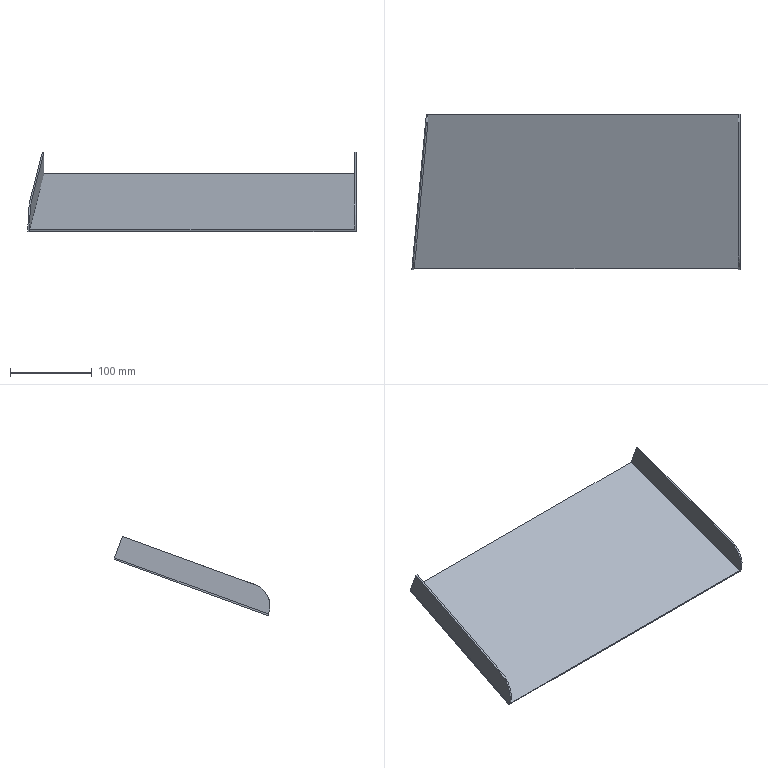Part | NX | features solid 2 | 1 solid | 16 faces | box 400.679 x 190.481 x 96.654 mm | volume 178538 mm3 | plane 11 | spline 3 | cylinder 2 | commonest cylinder face diameters 56 x2
STEP:
#1=CARTESIAN_POINT('',(-874.402,-997.254,-367.866));
#2=VERTEX_POINT('',#1);
#3=CARTESIAN_POINT('',(-475.731,-997.254,-367.866));
#4=VERTEX_POINT('',#3);
#5=CARTESIAN_POINT('',(-849.475,-997.254,-367.866));
#6=DIRECTION('',(-1.,0.,0.));
#7=VECTOR('',#6,1000.);
#8=LINE('',#5,#7);
#9=EDGE_CURVE('',#2,#4,#8,.F.);
#10=ORIENTED_EDGE('',*,*,#9,.T.);
#11=CARTESIAN_POINT('',(-475.731,-997.939,-365.986));
#12=VERTEX_POINT('',#11);
#13=CARTESIAN_POINT('',(-475.731,-997.254,-367.866));
#14=DIRECTION('',(0.,-0.342,0.9397));
#15=VECTOR('',#14,1000.);
#16=LINE('',#13,#15);
#17=EDGE_CURVE('',#4,#12,#16,.T.);
#18=ORIENTED_EDGE('',*,*,#17,.T.);
#19=CARTESIAN_POINT('',(-477.731,-997.939,-365.986));
#20=VERTEX_POINT('',#19);
#21=CARTESIAN_POINT('',(-475.731,-997.939,-365.986));
#22=DIRECTION('',(-1.,0.,0.));
#23=VECTOR('',#22,1000.);
#24=LINE('',#21,#23);
#25=EDGE_CURVE('',#12,#20,#24,.T.);
#26=ORIENTED_EDGE('',*,*,#25,.T.);
#27=CARTESIAN_POINT('',(-874.402,-997.939,-365.986));
#28=VERTEX_POINT('',#27);
#29=CARTESIAN_POINT('',(-849.475,-997.939,-365.986));
#30=DIRECTION('',(-1.,0.,0.));
#31=VECTOR('',#30,1000.);
#32=LINE('',#29,#31);
#33=EDGE_CURVE('',#28,#20,#32,.F.);
#34=ORIENTED_EDGE('',*,*,#33,.F.);
#35=CARTESIAN_POINT('',(-874.402,-997.254,-367.866));
#36=DIRECTION('',(0.,-0.342,0.9397));
#37=VECTOR('',#36,1000.);
#38=LINE('',#35,#37);
#39=EDGE_CURVE('',#28,#2,#38,.F.);
#40=ORIENTED_EDGE('',*,*,#39,.T.);
#41=EDGE_LOOP('',(#10,#18,#26,#34,#40));
#42=FACE_BOUND('',#41,.T.);
#43=CARTESIAN_POINT('',(-849.475,-997.254,-367.866));
#44=DIRECTION('',(0.,0.9397,0.342));
#45=DIRECTION('',(1.,0.,0.));
#46=AXIS2_PLACEMENT_3D('',#43,#44,#45);
#47=PLANE('',#46);
#48=ADVANCED_FACE('',(#42),#47,.F.);
#49=CARTESIAN_POINT('',(-858.894,-810.,-297.582));
#50=VERTEX_POINT('',#49);
#51=CARTESIAN_POINT('',(-477.731,-810.,-297.582));
#52=VERTEX_POINT('',#51);
#53=CARTESIAN_POINT('',(-849.475,-810.,-297.582));
#54=DIRECTION('',(1.,0.,0.));
#55=VECTOR('',#54,1000.);
#56=LINE('',#53,#55);
#57=EDGE_CURVE('',#50,#52,#56,.T.);
#58=ORIENTED_EDGE('',*,*,#57,.T.);
#59=CARTESIAN_POINT('',(-477.731,-819.577,-271.271));
#60=VERTEX_POINT('',#59);
#61=CARTESIAN_POINT('',(-477.731,-809.316,-299.462));
#62=DIRECTION('',(0.,-0.342,0.9397));
#63=VECTOR('',#62,1000.);
#64=LINE('',#61,#63);
#65=EDGE_CURVE('',#52,#60,#64,.T.);
#66=ORIENTED_EDGE('',*,*,#65,.T.);
#67=CARTESIAN_POINT('',(-475.731,-819.577,-271.271));
#68=VERTEX_POINT('',#67);
#69=CARTESIAN_POINT('',(-475.731,-819.577,-271.271));
#70=DIRECTION('',(1.,0.,0.));
#71=VECTOR('',#70,1000.);
#72=LINE('',#69,#71);
#73=EDGE_CURVE('',#68,#60,#72,.F.);
#74=ORIENTED_EDGE('',*,*,#73,.F.);
#75=CARTESIAN_POINT('',(-475.731,-809.316,-299.462));
#76=VERTEX_POINT('',#75);
#77=CARTESIAN_POINT('',(-475.731,-891.114,-74.722));
#78=DIRECTION('',(0.,0.342,-0.9397));
#79=VECTOR('',#78,1000.);
#80=LINE('',#77,#79);
#81=EDGE_CURVE('',#76,#68,#80,.F.);
#82=ORIENTED_EDGE('',*,*,#81,.F.);
#83=CARTESIAN_POINT('',(-858.894,-809.316,-299.462));
#84=VERTEX_POINT('',#83);
#85=CARTESIAN_POINT('',(-849.475,-809.316,-299.462));
#86=DIRECTION('',(1.,0.,0.));
#87=VECTOR('',#86,1000.);
#88=LINE('',#85,#87);
#89=EDGE_CURVE('',#84,#76,#88,.T.);
#90=ORIENTED_EDGE('',*,*,#89,.F.);
#91=CARTESIAN_POINT('',(-858.894,-809.658,-298.522));
#92=DIRECTION('',(0.,-0.342,0.9397));
#93=VECTOR('',#92,1000.);
#94=LINE('',#91,#93);
#95=EDGE_CURVE('',#84,#50,#94,.T.);
#96=ORIENTED_EDGE('',*,*,#95,.T.);
#97=EDGE_LOOP('',(#58,#66,#74,#82,#90,#96));
#98=FACE_BOUND('',#97,.T.);
#99=CARTESIAN_POINT('',(-849.475,-809.316,-299.462));
#100=DIRECTION('',(0.,0.9397,0.342));
#101=DIRECTION('',(1.,0.,0.));
#102=AXIS2_PLACEMENT_3D('',#99,#100,#101);
#103=PLANE('',#102);
#104=ADVANCED_FACE('',(#98),#103,.T.);
#105=ORIENTED_EDGE('',*,*,#95,.F.);
#106=CARTESIAN_POINT('',(-876.41,-997.254,-367.866));
#107=VERTEX_POINT('',#106);
#108=CARTESIAN_POINT('',(-858.894,-809.316,-299.462));
#109=CARTESIAN_POINT('',(-864.732,-871.962,-322.263));
#110=CARTESIAN_POINT('',(-870.571,-934.608,-345.064));
#111=CARTESIAN_POINT('',(-876.41,-997.254,-367.866));
#112=B_SPLINE_CURVE_WITH_KNOTS('',3,(#108,#109,#110,#111),.UNSPECIFIED.,.F.,.F.,(4,4),(-0.03011,0.1707),.UNSPECIFIED.);
#113=EDGE_CURVE('',#84,#107,#112,.T.);
#114=ORIENTED_EDGE('',*,*,#113,.T.);
#115=CARTESIAN_POINT('',(-876.41,-997.939,-365.986));
#116=VERTEX_POINT('',#115);
#117=CARTESIAN_POINT('',(-876.41,-997.597,-366.926));
#118=DIRECTION('',(0.,-0.342,0.9397));
#119=VECTOR('',#118,1000.);
#120=LINE('',#117,#119);
#121=EDGE_CURVE('',#107,#116,#120,.T.);
#122=ORIENTED_EDGE('',*,*,#121,.T.);
#123=CARTESIAN_POINT('',(-876.41,-997.939,-365.986));
#124=CARTESIAN_POINT('',(-870.571,-935.292,-343.185));
#125=CARTESIAN_POINT('',(-864.732,-872.646,-320.384));
#126=CARTESIAN_POINT('',(-858.894,-810.,-297.582));
#127=B_SPLINE_CURVE_WITH_KNOTS('',3,(#123,#124,#125,#126),.UNSPECIFIED.,.F.,.F.,(4,4),(0.6901,0.8909),.UNSPECIFIED.);
#128=EDGE_CURVE('',#50,#116,#127,.F.);
#129=ORIENTED_EDGE('',*,*,#128,.F.);
#130=EDGE_LOOP('',(#105,#114,#122,#129));
#131=FACE_BOUND('',#130,.T.);
#132=CARTESIAN_POINT('',(-858.894,-809.316,-299.462));
#133=CARTESIAN_POINT('',(-858.894,-810.,-297.582));
#134=CARTESIAN_POINT('',(-864.732,-871.962,-322.263));
#135=CARTESIAN_POINT('',(-864.732,-872.646,-320.384));
#136=CARTESIAN_POINT('',(-870.571,-934.608,-345.064));
#137=CARTESIAN_POINT('',(-870.571,-935.292,-343.185));
#138=CARTESIAN_POINT('',(-876.41,-997.254,-367.866));
#139=CARTESIAN_POINT('',(-876.41,-997.939,-365.986));
#140=B_SPLINE_SURFACE_WITH_KNOTS('',3,1,((#132,#133),(#134,#135),(#136,#137),(#138,#139)),.SURF_OF_LINEAR_EXTRUSION.,.F.,.F.,.F.,(4,4),(2,2),(0.,1.),(0.,1.),.PIECEWISE_BEZIER_KNOTS.);
#141=ADVANCED_FACE('',(#131),#140,.T.);
#142=ORIENTED_EDGE('',*,*,#33,.T.);
#143=CARTESIAN_POINT('',(-477.731,-838.191,-307.843));
#144=DIRECTION('',(0.,0.9397,0.342));
#145=VECTOR('',#144,1000.);
#146=LINE('',#143,#145);
#147=EDGE_CURVE('',#20,#52,#146,.T.);
#148=ORIENTED_EDGE('',*,*,#147,.T.);
#149=ORIENTED_EDGE('',*,*,#57,.F.);
#150=CARTESIAN_POINT('',(-856.901,-810.164,-297.642));
#151=VERTEX_POINT('',#150);
#152=CARTESIAN_POINT('',(-846.94,-810.984,-297.94));
#153=DIRECTION('',(-0.9962,0.08198,0.02984));
#154=VECTOR('',#153,1000.);
#155=LINE('',#152,#154);
#156=EDGE_CURVE('',#50,#151,#155,.F.);
#157=ORIENTED_EDGE('',*,*,#156,.T.);
#158=CARTESIAN_POINT('',(-859.437,-837.371,-307.545));
#159=DIRECTION('',(0.08725,0.9361,0.3407));
#160=VECTOR('',#159,1000.);
#161=LINE('',#158,#160);
#162=EDGE_CURVE('',#28,#151,#161,.T.);
#163=ORIENTED_EDGE('',*,*,#162,.F.);
#164=EDGE_LOOP('',(#142,#148,#149,#157,#163));
#165=FACE_BOUND('',#164,.T.);
#166=CARTESIAN_POINT('',(-849.475,-838.191,-307.843));
#167=DIRECTION('',(0.,0.342,-0.9397));
#168=DIRECTION('',(-1.,0.,0.));
#169=AXIS2_PLACEMENT_3D('',#166,#167,#168);
#170=PLANE('',#169);
#171=ADVANCED_FACE('',(#165),#170,.F.);
#172=CARTESIAN_POINT('',(-475.731,-837.507,-309.722));
#173=DIRECTION('',(0.,0.9397,0.342));
#174=VECTOR('',#173,1000.);
#175=LINE('',#172,#174);
#176=EDGE_CURVE('',#76,#4,#175,.F.);
#177=ORIENTED_EDGE('',*,*,#176,.F.);
#178=ORIENTED_EDGE('',*,*,#81,.T.);
#179=CARTESIAN_POINT('',(-475.731,-981.204,-330.098));
#180=VERTEX_POINT('',#179);
#181=CARTESIAN_POINT('',(-475.731,-819.577,-271.271));
#182=DIRECTION('',(0.,-0.9397,-0.342));
#183=VECTOR('',#182,1000.);
#184=LINE('',#181,#183);
#185=EDGE_CURVE('',#68,#180,#184,.T.);
#186=ORIENTED_EDGE('',*,*,#185,.T.);
#187=CARTESIAN_POINT('',(-475.731,-971.627,-356.41));
#188=DIRECTION('',(-1.,0.,0.));
#189=DIRECTION('',(0.,-1.,0.));
#190=AXIS2_PLACEMENT_3D('',#187,#188,#189);
#191=CIRCLE('',#190,28.);
#192=EDGE_CURVE('',#180,#12,#191,.F.);
#193=ORIENTED_EDGE('',*,*,#192,.T.);
#194=ORIENTED_EDGE('',*,*,#17,.F.);
#195=EDGE_LOOP('',(#177,#178,#186,#193,#194));
#196=FACE_BOUND('',#195,.T.);
#197=CARTESIAN_POINT('',(-475.731,-608.443,28.162));
#198=DIRECTION('',(-1.,0.,0.));
#199=DIRECTION('',(0.,-0.9397,-0.342));
#200=AXIS2_PLACEMENT_3D('',#197,#198,#199);
#201=PLANE('',#200);
#202=ADVANCED_FACE('',(#196),#201,.F.);
#203=ORIENTED_EDGE('',*,*,#89,.T.);
#204=ORIENTED_EDGE('',*,*,#176,.T.);
#205=ORIENTED_EDGE('',*,*,#9,.F.);
#206=CARTESIAN_POINT('',(-876.41,-997.254,-367.866));
#207=VERTEX_POINT('',#206);
#208=CARTESIAN_POINT('',(-849.475,-997.254,-367.866));
#209=DIRECTION('',(-1.,0.,0.));
#210=VECTOR('',#209,1000.);
#211=LINE('',#208,#210);
#212=EDGE_CURVE('',#207,#2,#211,.F.);
#213=ORIENTED_EDGE('',*,*,#212,.F.);
#214=CARTESIAN_POINT('',(-849.475,-997.254,-367.866));
#215=DIRECTION('',(-1.,0.,0.));
#216=VECTOR('',#215,1000.);
#217=LINE('',#214,#216);
#218=EDGE_CURVE('',#107,#207,#217,.F.);
#219=ORIENTED_EDGE('',*,*,#218,.F.);
#220=ORIENTED_EDGE('',*,*,#113,.F.);
#221=EDGE_LOOP('',(#203,#204,#205,#213,#219,#220));
#222=FACE_BOUND('',#221,.T.);
#223=CARTESIAN_POINT('',(-849.475,-837.507,-309.722));
#224=DIRECTION('',(0.,0.342,-0.9397));
#225=DIRECTION('',(-1.,0.,0.));
#226=AXIS2_PLACEMENT_3D('',#223,#224,#225);
#227=PLANE('',#226);
#228=ADVANCED_FACE('',(#222),#227,.T.);
#229=ORIENTED_EDGE('',*,*,#156,.F.);
#230=CARTESIAN_POINT('',(-858.894,-819.577,-271.271));
#231=VERTEX_POINT('',#230);
#232=CARTESIAN_POINT('',(-858.894,-809.316,-299.462));
#233=DIRECTION('',(0.,-0.342,0.9397));
#234=VECTOR('',#233,1000.);
#235=LINE('',#232,#234);
#236=EDGE_CURVE('',#50,#231,#235,.T.);
#237=ORIENTED_EDGE('',*,*,#236,.T.);
#238=CARTESIAN_POINT('',(-856.901,-819.741,-271.331));
#239=VERTEX_POINT('',#238);
#240=CARTESIAN_POINT('',(-858.894,-819.577,-271.271));
#241=DIRECTION('',(0.9962,-0.08198,-0.02984));
#242=VECTOR('',#241,1000.);
#243=LINE('',#240,#242);
#244=EDGE_CURVE('',#231,#239,#243,.T.);
#245=ORIENTED_EDGE('',*,*,#244,.T.);
#246=CARTESIAN_POINT('',(-856.901,-809.48,-299.521));
#247=DIRECTION('',(0.,-0.342,0.9397));
#248=VECTOR('',#247,1000.);
#249=LINE('',#246,#248);
#250=EDGE_CURVE('',#151,#239,#249,.T.);
#251=ORIENTED_EDGE('',*,*,#250,.F.);
#252=EDGE_LOOP('',(#229,#237,#245,#251));
#253=FACE_BOUND('',#252,.T.);
#254=CARTESIAN_POINT('',(-858.894,-809.316,-299.462));
#255=DIRECTION('',(-0.08725,-0.9361,-0.3407));
#256=DIRECTION('',(0.,-0.342,0.9397));
#257=AXIS2_PLACEMENT_3D('',#254,#255,#256);
#258=PLANE('',#257);
#259=ADVANCED_FACE('',(#253),#258,.F.);
#260=ORIENTED_EDGE('',*,*,#128,.T.);
#261=CARTESIAN_POINT('',(-873.967,-981.304,-330.135));
#262=VERTEX_POINT('',#261);
#263=CARTESIAN_POINT('',(-873.967,-971.727,-356.446));
#264=DIRECTION('',(-0.9962,0.08198,0.02984));
#265=DIRECTION('',(-0.08202,-0.9966,0.));
#266=AXIS2_PLACEMENT_3D('',#263,#264,#265);
#267=CIRCLE('',#266,28.);
#268=EDGE_CURVE('',#116,#262,#267,.T.);
#269=ORIENTED_EDGE('',*,*,#268,.T.);
#270=CARTESIAN_POINT('',(-858.894,-819.577,-271.271));
#271=CARTESIAN_POINT('',(-864.732,-882.223,-294.072));
#272=CARTESIAN_POINT('',(-870.571,-944.869,-316.874));
#273=CARTESIAN_POINT('',(-876.41,-1007.515,-339.675));
#274=B_SPLINE_CURVE_WITH_KNOTS('',3,(#270,#271,#272,#273),.UNSPECIFIED.,.F.,.F.,(4,4),(0.,1.),.PIECEWISE_BEZIER_KNOTS.);
#275=EDGE_CURVE('',#231,#262,#274,.T.);
#276=ORIENTED_EDGE('',*,*,#275,.F.);
#277=ORIENTED_EDGE('',*,*,#236,.F.);
#278=EDGE_LOOP('',(#260,#269,#276,#277));
#279=FACE_BOUND('',#278,.T.);
#280=CARTESIAN_POINT('',(-858.894,-809.316,-299.462));
#281=DIRECTION('',(-0.9962,0.08198,0.02984));
#282=DIRECTION('',(-0.08202,-0.9966,0.));
#283=AXIS2_PLACEMENT_3D('',#280,#281,#282);
#284=PLANE('',#283);
#285=ADVANCED_FACE('',(#279),#284,.T.);
#286=CARTESIAN_POINT('',(-874.417,-997.418,-367.925));
#287=VERTEX_POINT('',#286);
#288=CARTESIAN_POINT('',(-876.41,-997.254,-367.866));
#289=DIRECTION('',(0.9962,-0.08198,-0.02984));
#290=VECTOR('',#289,1000.);
#291=LINE('',#288,#290);
#292=EDGE_CURVE('',#207,#287,#291,.T.);
#293=ORIENTED_EDGE('',*,*,#292,.F.);
#294=ORIENTED_EDGE('',*,*,#212,.T.);
#295=CARTESIAN_POINT('',(-856.901,-809.48,-299.521));
#296=CARTESIAN_POINT('',(-862.74,-872.126,-322.323));
#297=CARTESIAN_POINT('',(-868.579,-934.772,-345.124));
#298=CARTESIAN_POINT('',(-874.417,-997.418,-367.925));
#299=B_SPLINE_CURVE_WITH_KNOTS('',3,(#295,#296,#297,#298),.UNSPECIFIED.,.F.,.F.,(4,4),(0.,1.),.UNSPECIFIED.);
#300=EDGE_CURVE('',#2,#287,#299,.T.);
#301=ORIENTED_EDGE('',*,*,#300,.T.);
#302=EDGE_LOOP('',(#293,#294,#301));
#303=FACE_BOUND('',#302,.T.);
#304=CARTESIAN_POINT('',(-874.402,-997.254,-367.865));
#305=CARTESIAN_POINT('',(-876.406,-997.089,-367.805));
#306=CARTESIAN_POINT('',(-874.407,-997.308,-367.885));
#307=CARTESIAN_POINT('',(-876.411,-997.144,-367.825));
#308=CARTESIAN_POINT('',(-874.412,-997.363,-367.905));
#309=CARTESIAN_POINT('',(-876.417,-997.199,-367.845));
#310=CARTESIAN_POINT('',(-874.417,-997.418,-367.925));
#311=CARTESIAN_POINT('',(-876.422,-997.254,-367.865));
#312=B_SPLINE_SURFACE_WITH_KNOTS('',3,1,((#304,#305),(#306,#307),(#308,#309),(#310,#311)),.SURF_OF_LINEAR_EXTRUSION.,.F.,.F.,.F.,(4,4),(2,2),(0.9991,1.),(0.,1.),.PIECEWISE_BEZIER_KNOTS.);
#313=ADVANCED_FACE('',(#303),#312,.T.);
#314=ORIENTED_EDGE('',*,*,#275,.T.);
#315=CARTESIAN_POINT('',(-871.975,-981.468,-330.195));
#316=VERTEX_POINT('',#315);
#317=CARTESIAN_POINT('',(-873.967,-981.304,-330.135));
#318=DIRECTION('',(-0.9962,0.08198,0.02984));
#319=VECTOR('',#318,1000.);
#320=LINE('',#317,#319);
#321=EDGE_CURVE('',#262,#316,#320,.F.);
#322=ORIENTED_EDGE('',*,*,#321,.T.);
#323=CARTESIAN_POINT('',(-856.901,-819.741,-271.331));
#324=CARTESIAN_POINT('',(-862.74,-882.387,-294.132));
#325=CARTESIAN_POINT('',(-868.579,-945.033,-316.933));
#326=CARTESIAN_POINT('',(-874.417,-1007.679,-339.735));
#327=B_SPLINE_CURVE_WITH_KNOTS('',3,(#323,#324,#325,#326),.UNSPECIFIED.,.F.,.F.,(4,4),(0.,1.),.UNSPECIFIED.);
#328=EDGE_CURVE('',#239,#316,#327,.T.);
#329=ORIENTED_EDGE('',*,*,#328,.F.);
#330=ORIENTED_EDGE('',*,*,#244,.F.);
#331=EDGE_LOOP('',(#314,#322,#329,#330));
#332=FACE_BOUND('',#331,.T.);
#333=CARTESIAN_POINT('',(-856.901,-819.741,-271.331));
#334=CARTESIAN_POINT('',(-858.894,-819.577,-271.271));
#335=CARTESIAN_POINT('',(-861.926,-873.65,-290.952));
#336=CARTESIAN_POINT('',(-863.918,-873.486,-290.892));
#337=CARTESIAN_POINT('',(-866.95,-927.559,-310.573));
#338=CARTESIAN_POINT('',(-868.943,-927.395,-310.514));
#339=CARTESIAN_POINT('',(-871.975,-981.468,-330.195));
#340=CARTESIAN_POINT('',(-873.967,-981.304,-330.135));
#341=B_SPLINE_SURFACE_WITH_KNOTS('',3,1,((#333,#334),(#335,#336),(#337,#338),(#339,#340)),.SURF_OF_LINEAR_EXTRUSION.,.F.,.F.,.F.,(4,4),(2,2),(0.,0.8605),(0.,1.),.PIECEWISE_BEZIER_KNOTS.);
#342=ADVANCED_FACE('',(#332),#341,.F.);
#343=ORIENTED_EDGE('',*,*,#39,.F.);
#344=ORIENTED_EDGE('',*,*,#162,.T.);
#345=ORIENTED_EDGE('',*,*,#250,.T.);
#346=ORIENTED_EDGE('',*,*,#328,.T.);
#347=CARTESIAN_POINT('',(-874.417,-998.102,-366.046));
#348=VERTEX_POINT('',#347);
#349=CARTESIAN_POINT('',(-871.975,-971.891,-356.506));
#350=DIRECTION('',(-0.9962,0.08198,0.02984));
#351=DIRECTION('',(-0.08202,-0.9966,0.));
#352=AXIS2_PLACEMENT_3D('',#349,#350,#351);
#353=CIRCLE('',#352,28.);
#354=EDGE_CURVE('',#316,#348,#353,.F.);
#355=ORIENTED_EDGE('',*,*,#354,.T.);
#356=CARTESIAN_POINT('',(-874.417,-997.418,-367.925));
#357=DIRECTION('',(0.,-0.342,0.9397));
#358=VECTOR('',#357,1000.);
#359=LINE('',#356,#358);
#360=EDGE_CURVE('',#287,#348,#359,.T.);
#361=ORIENTED_EDGE('',*,*,#360,.F.);
#362=ORIENTED_EDGE('',*,*,#300,.F.);
#363=EDGE_LOOP('',(#343,#344,#345,#346,#355,#361,#362));
#364=FACE_BOUND('',#363,.T.);
#365=CARTESIAN_POINT('',(-856.901,-809.48,-299.521));
#366=DIRECTION('',(-0.9962,0.08198,0.02984));
#367=DIRECTION('',(-0.08202,-0.9966,0.));
#368=AXIS2_PLACEMENT_3D('',#365,#366,#367);
#369=PLANE('',#368);
#370=ADVANCED_FACE('',(#364),#369,.F.);
#371=ORIENTED_EDGE('',*,*,#360,.T.);
#372=CARTESIAN_POINT('',(-876.41,-997.939,-365.986));
#373=DIRECTION('',(-0.9962,0.08198,0.02984));
#374=VECTOR('',#373,1000.);
#375=LINE('',#372,#374);
#376=EDGE_CURVE('',#348,#116,#375,.T.);
#377=ORIENTED_EDGE('',*,*,#376,.T.);
#378=ORIENTED_EDGE('',*,*,#121,.F.);
#379=ORIENTED_EDGE('',*,*,#218,.T.);
#380=ORIENTED_EDGE('',*,*,#292,.T.);
#381=EDGE_LOOP('',(#371,#377,#378,#379,#380));
#382=FACE_BOUND('',#381,.T.);
#383=CARTESIAN_POINT('',(-876.41,-997.254,-367.866));
#384=DIRECTION('',(-0.08725,-0.9361,-0.3407));
#385=DIRECTION('',(0.,-0.342,0.9397));
#386=AXIS2_PLACEMENT_3D('',#383,#384,#385);
#387=PLANE('',#386);
#388=ADVANCED_FACE('',(#382),#387,.T.);
#389=ORIENTED_EDGE('',*,*,#268,.F.);
#390=ORIENTED_EDGE('',*,*,#376,.F.);
#391=ORIENTED_EDGE('',*,*,#354,.F.);
#392=ORIENTED_EDGE('',*,*,#321,.F.);
#393=EDGE_LOOP('',(#389,#390,#391,#392));
#394=FACE_BOUND('',#393,.T.);
#395=CARTESIAN_POINT('',(-872.971,-971.809,-356.476));
#396=DIRECTION('',(-0.9962,0.08198,0.02984));
#397=DIRECTION('',(-0.08202,-0.9966,0.));
#398=AXIS2_PLACEMENT_3D('',#395,#396,#397);
#399=CYLINDRICAL_SURFACE('',#398,28.);
#400=ADVANCED_FACE('',(#394),#399,.T.);
#401=ORIENTED_EDGE('',*,*,#147,.F.);
#402=CARTESIAN_POINT('',(-477.731,-981.204,-330.098));
#403=VERTEX_POINT('',#402);
#404=CARTESIAN_POINT('',(-477.731,-971.627,-356.41));
#405=DIRECTION('',(-1.,0.,0.));
#406=DIRECTION('',(0.,-1.,0.));
#407=AXIS2_PLACEMENT_3D('',#404,#405,#406);
#408=CIRCLE('',#407,28.);
#409=EDGE_CURVE('',#20,#403,#408,.T.);
#410=ORIENTED_EDGE('',*,*,#409,.T.);
#411=CARTESIAN_POINT('',(-477.731,-819.577,-271.271));
#412=DIRECTION('',(0.,-0.9397,-0.342));
#413=VECTOR('',#412,1000.);
#414=LINE('',#411,#413);
#415=EDGE_CURVE('',#60,#403,#414,.T.);
#416=ORIENTED_EDGE('',*,*,#415,.F.);
#417=ORIENTED_EDGE('',*,*,#65,.F.);
#418=EDGE_LOOP('',(#401,#410,#416,#417));
#419=FACE_BOUND('',#418,.T.);
#420=CARTESIAN_POINT('',(-477.731,-809.316,-299.462));
#421=DIRECTION('',(-1.,0.,0.));
#422=DIRECTION('',(0.,-1.,0.));
#423=AXIS2_PLACEMENT_3D('',#420,#421,#422);
#424=PLANE('',#423);
#425=ADVANCED_FACE('',(#419),#424,.T.);
#426=ORIENTED_EDGE('',*,*,#415,.T.);
#427=CARTESIAN_POINT('',(-475.731,-981.204,-330.098));
#428=DIRECTION('',(1.,0.,0.));
#429=VECTOR('',#428,1000.);
#430=LINE('',#427,#429);
#431=EDGE_CURVE('',#403,#180,#430,.T.);
#432=ORIENTED_EDGE('',*,*,#431,.T.);
#433=ORIENTED_EDGE('',*,*,#185,.F.);
#434=ORIENTED_EDGE('',*,*,#73,.T.);
#435=EDGE_LOOP('',(#426,#432,#433,#434));
#436=FACE_BOUND('',#435,.T.);
#437=CARTESIAN_POINT('',(-475.731,-819.577,-271.271));
#438=DIRECTION('',(0.,0.342,-0.9397));
#439=DIRECTION('',(0.,-0.9397,-0.342));
#440=AXIS2_PLACEMENT_3D('',#437,#438,#439);
#441=PLANE('',#440);
#442=ADVANCED_FACE('',(#436),#441,.F.);
#443=ORIENTED_EDGE('',*,*,#192,.F.);
#444=ORIENTED_EDGE('',*,*,#431,.F.);
#445=ORIENTED_EDGE('',*,*,#409,.F.);
#446=ORIENTED_EDGE('',*,*,#25,.F.);
#447=EDGE_LOOP('',(#443,#444,#445,#446));
#448=FACE_BOUND('',#447,.T.);
#449=CARTESIAN_POINT('',(-475.731,-971.627,-356.41));
#450=DIRECTION('',(1.,0.,0.));
#451=DIRECTION('',(0.,1.,0.));
#452=AXIS2_PLACEMENT_3D('',#449,#450,#451);
#453=CYLINDRICAL_SURFACE('',#452,28.);
#454=ADVANCED_FACE('',(#448),#453,.T.);
#455=CLOSED_SHELL('',(#48,#104,#141,#171,#202,#228,#259,#285,#313,#342,#370,#388,#400,#425,#442,#454));
#456=MANIFOLD_SOLID_BREP('',#455);
#457=(LENGTH_UNIT()NAMED_UNIT(*)SI_UNIT(.MILLI.,.METRE.));
#458=UNCERTAINTY_MEASURE_WITH_UNIT(LENGTH_MEASURE(0.0508),#457,'','');
#459=(NAMED_UNIT(*)PLANE_ANGLE_UNIT()SI_UNIT($,.RADIAN.));
#460=(NAMED_UNIT(*)SI_UNIT($,.STERADIAN.)SOLID_ANGLE_UNIT());
#461=(GEOMETRIC_REPRESENTATION_CONTEXT(3)GLOBAL_UNCERTAINTY_ASSIGNED_CONTEXT((#458))GLOBAL_UNIT_ASSIGNED_CONTEXT((#457,#459,#460))REPRESENTATION_CONTEXT('',''));
#462=ADVANCED_BREP_SHAPE_REPRESENTATION('',(#456),#461);